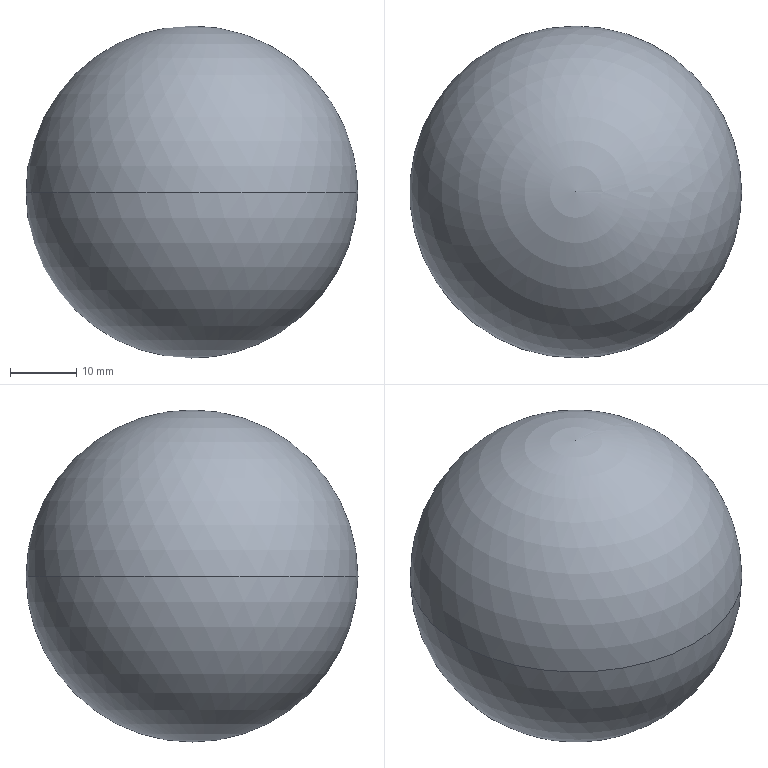Part | SolidWorks | features Revolution 1 | 1 solid | 2 faces | box 50 x 50 x 50 mm | volume 65450 mm3 | sphere 2
STEP:
#1=CARTESIAN_POINT('',(0.,-25.,0.));
#2=VERTEX_POINT('',#1);
#3=CARTESIAN_POINT('',(0.,25.,0.));
#4=VERTEX_POINT('',#3);
#5=CARTESIAN_POINT('',(0.,0.,0.));
#6=DIRECTION('',(0.,0.,1.));
#7=DIRECTION('',(1.,0.,0.));
#8=AXIS2_PLACEMENT_3D('',#5,#6,#7);
#9=CIRCLE('',#8,25.);
#10=EDGE_CURVE('',#2,#4,#9,.T.);
#11=ORIENTED_EDGE('',*,*,#10,.F.);
#12=CARTESIAN_POINT('',(0.,0.,0.));
#13=DIRECTION('',(0.,0.,-1.));
#14=DIRECTION('',(-1.,0.,0.));
#15=AXIS2_PLACEMENT_3D('',#12,#13,#14);
#16=CIRCLE('',#15,25.);
#17=EDGE_CURVE('',#2,#4,#16,.T.);
#18=ORIENTED_EDGE('',*,*,#17,.T.);
#19=EDGE_LOOP('',(#11,#18));
#20=FACE_OUTER_BOUND('',#19,.T.);
#21=CARTESIAN_POINT('',(0.,0.,0.));
#22=DIRECTION('',(0.,0.,-1.));
#23=DIRECTION('',(1.,0.,0.));
#24=AXIS2_PLACEMENT_3D('',#21,#22,#23);
#25=SPHERICAL_SURFACE('',#24,25.);
#26=ADVANCED_FACE('',(#20),#25,.T.);
#27=ORIENTED_EDGE('',*,*,#17,.F.);
#28=ORIENTED_EDGE('',*,*,#10,.T.);
#29=EDGE_LOOP('',(#27,#28));
#30=FACE_OUTER_BOUND('',#29,.T.);
#31=CARTESIAN_POINT('',(0.,0.,0.));
#32=DIRECTION('',(0.,0.,-1.));
#33=DIRECTION('',(1.,0.,0.));
#34=AXIS2_PLACEMENT_3D('',#31,#32,#33);
#35=SPHERICAL_SURFACE('',#34,25.);
#36=ADVANCED_FACE('',(#30),#35,.T.);
#37=CLOSED_SHELL('',(#26,#36));
#38=MANIFOLD_SOLID_BREP('',#37);
#39=CARTESIAN_POINT('',(0.,0.,0.));
#40=DIRECTION('',(0.,0.,1.));
#41=DIRECTION('',(1.,0.,0.));
#42=AXIS2_PLACEMENT_3D('',#39,#40,#41);
#43=(LENGTH_UNIT()NAMED_UNIT(*)SI_UNIT(.MILLI.,.METRE.));
#44=UNCERTAINTY_MEASURE_WITH_UNIT(LENGTH_MEASURE(0.00001),#43,'','');
#45=(NAMED_UNIT(*)PLANE_ANGLE_UNIT()SI_UNIT($,.RADIAN.));
#46=(NAMED_UNIT(*)SI_UNIT($,.STERADIAN.)SOLID_ANGLE_UNIT());
#47=(GEOMETRIC_REPRESENTATION_CONTEXT(3)GLOBAL_UNCERTAINTY_ASSIGNED_CONTEXT((#44))GLOBAL_UNIT_ASSIGNED_CONTEXT((#43,#45,#46))REPRESENTATION_CONTEXT('',''));
#48=ADVANCED_BREP_SHAPE_REPRESENTATION('',(#38,#42),#47);